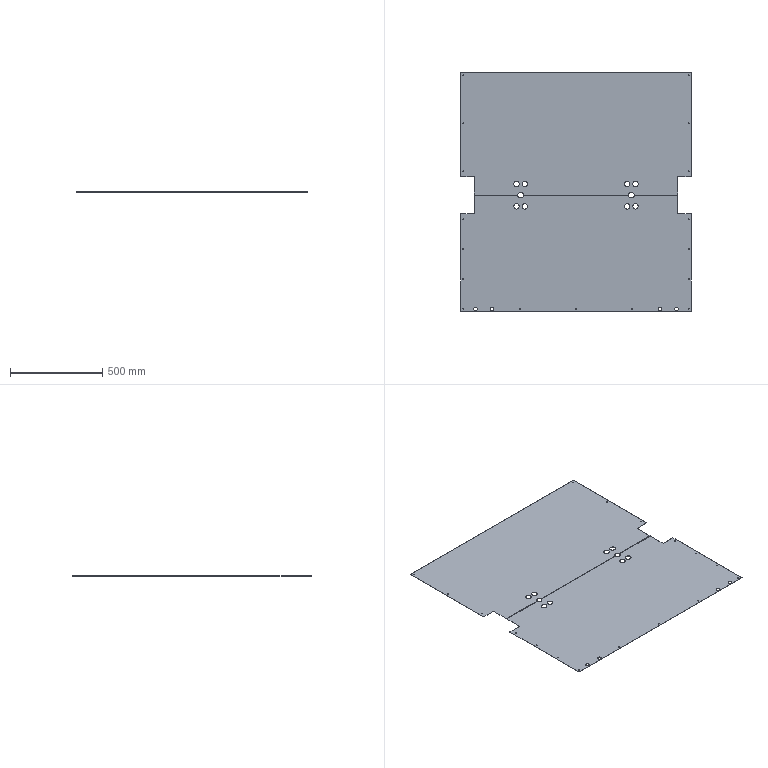Part | 2 solids | 88 faces | box 1250 x 1295 x 1 mm | volume 1578009 mm3 | cylinder 64 | plane 24 | commonest cylinder face diameters 5 x34 30 x20 20 x8 4 x2